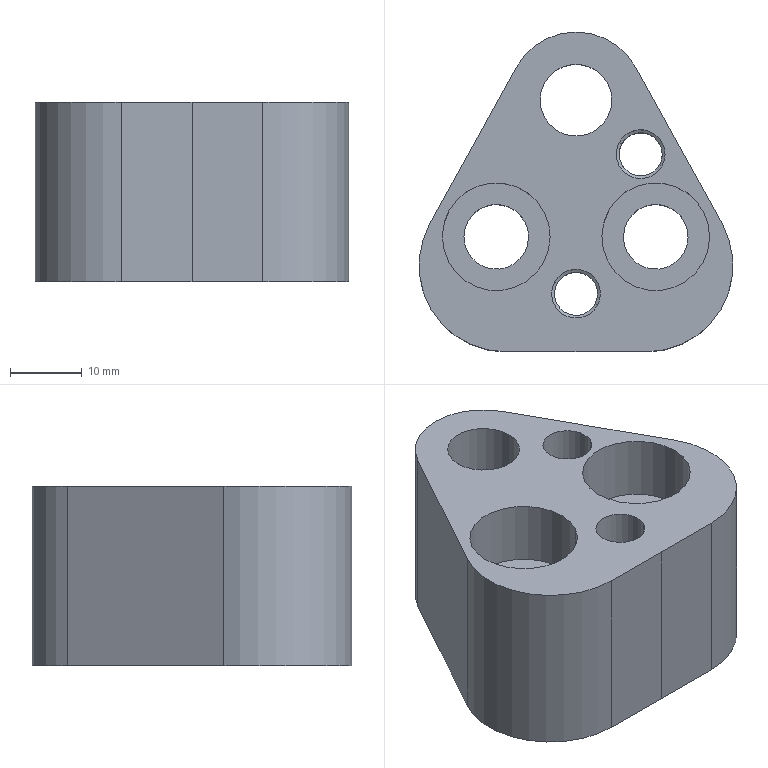Part | CATIA | 1 solid | 42 faces | box 43.7 x 44.5 x 25 mm | volume 25763 mm3 | cylinder 26 | plane 12 | cone 4 | commonest cylinder face diameters 6 x4 6.8 x4 9 x4 15 x4 5 x2 10 x2
STEP:
#1=CARTESIAN_POINT('',(2.984,-28.56,25.));
#2=VERTEX_POINT('',#1);
#3=CARTESIAN_POINT('',(-2.984,-25.3,25.));
#4=VERTEX_POINT('',#3);
#5=CARTESIAN_POINT('',(0.,-26.93,25.));
#6=DIRECTION('',(0.,0.,-1.));
#7=AXIS2_PLACEMENT_3D('',#5,#6,$);
#8=CIRCLE('',#7,3.4);
#9=EDGE_CURVE('',#2,#4,#8,.F.);
#10=ORIENTED_EDGE('',*,*,#9,.T.);
#11=CARTESIAN_POINT('',(-2.984,-25.3,16.));
#12=VERTEX_POINT('',#11);
#13=CARTESIAN_POINT('',(-2.984,-25.3,20.655));
#14=DIRECTION('',(0.,0.,-1.));
#15=VECTOR('',#14,1.);
#16=LINE('',#13,#15);
#17=EDGE_CURVE('',#12,#4,#16,.F.);
#18=ORIENTED_EDGE('',*,*,#17,.F.);
#19=CARTESIAN_POINT('',(2.984,-28.56,16.));
#20=VERTEX_POINT('',#19);
#21=CARTESIAN_POINT('',(0.,-26.93,16.));
#22=DIRECTION('',(0.,0.,-1.));
#23=AXIS2_PLACEMENT_3D('',#21,#22,$);
#24=CIRCLE('',#23,3.4);
#25=EDGE_CURVE('',#12,#20,#24,.T.);
#26=ORIENTED_EDGE('',*,*,#25,.T.);
#27=CARTESIAN_POINT('',(2.984,-28.56,20.655));
#28=DIRECTION('',(0.,0.,-1.));
#29=VECTOR('',#28,1.);
#30=LINE('',#27,#29);
#31=EDGE_CURVE('',#20,#2,#30,.F.);
#32=ORIENTED_EDGE('',*,*,#31,.T.);
#33=EDGE_LOOP('',(#10,#18,#26,#32));
#34=FACE_OUTER_BOUND('',#33,.T.);
#35=CARTESIAN_POINT('',(0.,-26.93,24.9));
#36=DIRECTION('',(0.,0.,-1.));
#37=DIRECTION('',(0.8776,-0.4794,0.));
#38=AXIS2_PLACEMENT_3D('',#35,#36,#37);
#39=CYLINDRICAL_SURFACE('',#38,3.4);
#40=ADVANCED_FACE('',(#34),#39,.F.);
#41=CARTESIAN_POINT('',(0.,-26.93,25.));
#42=DIRECTION('',(0.,0.,-1.));
#43=AXIS2_PLACEMENT_3D('',#41,#42,$);
#44=CIRCLE('',#43,3.4);
#45=EDGE_CURVE('',#4,#2,#44,.F.);
#46=ORIENTED_EDGE('',*,*,#45,.T.);
#47=ORIENTED_EDGE('',*,*,#31,.F.);
#48=CARTESIAN_POINT('',(0.,-26.93,16.));
#49=DIRECTION('',(0.,0.,-1.));
#50=AXIS2_PLACEMENT_3D('',#48,#49,$);
#51=CIRCLE('',#50,3.4);
#52=EDGE_CURVE('',#20,#12,#51,.T.);
#53=ORIENTED_EDGE('',*,*,#52,.T.);
#54=ORIENTED_EDGE('',*,*,#17,.T.);
#55=EDGE_LOOP('',(#46,#47,#53,#54));
#56=FACE_OUTER_BOUND('',#55,.T.);
#57=ADVANCED_FACE('',(#56),#39,.F.);
#58=CARTESIAN_POINT('',(-2.633,-25.492,15.769));
#59=VERTEX_POINT('',#58);
#60=CARTESIAN_POINT('',(3.,-26.93,15.769));
#61=VERTEX_POINT('',#60);
#62=CARTESIAN_POINT('',(0.,-26.93,15.769));
#63=DIRECTION('',(0.,0.,1.));
#64=AXIS2_PLACEMENT_3D('',#62,#63,$);
#65=CIRCLE('',#64,3.);
#66=EDGE_CURVE('',#59,#61,#65,.F.);
#67=ORIENTED_EDGE('',*,*,#66,.T.);
#68=CARTESIAN_POINT('',(2.633,-28.368,15.769));
#69=VERTEX_POINT('',#68);
#70=CARTESIAN_POINT('',(0.,-26.93,15.769));
#71=DIRECTION('',(0.,0.,1.));
#72=AXIS2_PLACEMENT_3D('',#70,#71,$);
#73=CIRCLE('',#72,3.);
#74=EDGE_CURVE('',#69,#61,#73,.T.);
#75=ORIENTED_EDGE('',*,*,#74,.F.);
#76=CARTESIAN_POINT('',(1.492,-27.745,15.019));
#77=DIRECTION('',(0.76,-0.4152,0.5));
#78=VECTOR('',#77,1.);
#79=LINE('',#76,#78);
#80=EDGE_CURVE('',#69,#20,#79,.T.);
#81=ORIENTED_EDGE('',*,*,#80,.T.);
#82=ORIENTED_EDGE('',*,*,#25,.F.);
#83=CARTESIAN_POINT('',(-1.492,-26.115,15.019));
#84=DIRECTION('',(-0.76,0.4152,0.5));
#85=VECTOR('',#84,1.);
#86=LINE('',#83,#85);
#87=EDGE_CURVE('',#59,#12,#86,.T.);
#88=ORIENTED_EDGE('',*,*,#87,.F.);
#89=EDGE_LOOP('',(#67,#75,#81,#82,#88));
#90=FACE_OUTER_BOUND('',#89,.T.);
#91=CARTESIAN_POINT('',(0.,-26.93,14.037));
#92=DIRECTION('',(0.,0.,1.));
#93=DIRECTION('',(0.8776,-0.4794,0.));
#94=AXIS2_PLACEMENT_3D('',#91,#92,#93);
#95=CONICAL_SURFACE('',#94,0.,1.047);
#96=ADVANCED_FACE('',(#90),#95,.F.);
#97=CARTESIAN_POINT('',(-3.,-26.93,15.769));
#98=VERTEX_POINT('',#97);
#99=CARTESIAN_POINT('',(0.,-26.93,15.769));
#100=DIRECTION('',(0.,0.,1.));
#101=AXIS2_PLACEMENT_3D('',#99,#100,$);
#102=CIRCLE('',#101,3.);
#103=EDGE_CURVE('',#69,#98,#102,.F.);
#104=ORIENTED_EDGE('',*,*,#103,.T.);
#105=CARTESIAN_POINT('',(0.,-26.93,15.769));
#106=DIRECTION('',(0.,0.,1.));
#107=AXIS2_PLACEMENT_3D('',#105,#106,$);
#108=CIRCLE('',#107,3.);
#109=EDGE_CURVE('',#59,#98,#108,.T.);
#110=ORIENTED_EDGE('',*,*,#109,.F.);
#111=ORIENTED_EDGE('',*,*,#87,.T.);
#112=ORIENTED_EDGE('',*,*,#52,.F.);
#113=ORIENTED_EDGE('',*,*,#80,.F.);
#114=EDGE_LOOP('',(#104,#110,#111,#112,#113));
#115=FACE_OUTER_BOUND('',#114,.T.);
#116=ADVANCED_FACE('',(#115),#95,.F.);
#117=ORIENTED_EDGE('',*,*,#66,.F.);
#118=ORIENTED_EDGE('',*,*,#109,.T.);
#119=CARTESIAN_POINT('',(-3.,-26.93,0.));
#120=VERTEX_POINT('',#119);
#121=CARTESIAN_POINT('',(-3.,-26.93,12.5));
#122=DIRECTION('',(0.,0.,1.));
#123=VECTOR('',#122,1.);
#124=LINE('',#121,#123);
#125=EDGE_CURVE('',#120,#98,#124,.T.);
#126=ORIENTED_EDGE('',*,*,#125,.F.);
#127=CARTESIAN_POINT('',(3.,-26.93,0.));
#128=VERTEX_POINT('',#127);
#129=CARTESIAN_POINT('',(0.,-26.93,0.));
#130=DIRECTION('',(0.,0.,1.));
#131=AXIS2_PLACEMENT_3D('',#129,#130,$);
#132=CIRCLE('',#131,3.);
#133=EDGE_CURVE('',#128,#120,#132,.T.);
#134=ORIENTED_EDGE('',*,*,#133,.F.);
#135=CARTESIAN_POINT('',(3.,-26.93,12.5));
#136=DIRECTION('',(0.,0.,1.));
#137=VECTOR('',#136,1.);
#138=LINE('',#135,#137);
#139=EDGE_CURVE('',#128,#61,#138,.T.);
#140=ORIENTED_EDGE('',*,*,#139,.T.);
#141=EDGE_LOOP('',(#117,#118,#126,#134,#140));
#142=FACE_OUTER_BOUND('',#141,.T.);
#143=CARTESIAN_POINT('',(0.,-26.93,12.5));
#144=DIRECTION('',(0.,0.,1.));
#145=DIRECTION('',(1.,0.,0.));
#146=AXIS2_PLACEMENT_3D('',#143,#144,#145);
#147=CYLINDRICAL_SURFACE('',#146,3.);
#148=ADVANCED_FACE('',(#142),#147,.F.);
#149=CARTESIAN_POINT('',(8.315,4.594,0.));
#150=VERTEX_POINT('',#149);
#151=CARTESIAN_POINT('',(8.315,4.594,25.));
#152=VERTEX_POINT('',#151);
#153=CARTESIAN_POINT('',(8.315,4.594,12.5));
#154=DIRECTION('',(0.,0.,1.));
#155=VECTOR('',#154,1.);
#156=LINE('',#153,#155);
#157=EDGE_CURVE('',#150,#152,#156,.T.);
#158=ORIENTED_EDGE('',*,*,#157,.F.);
#159=CARTESIAN_POINT('',(0.,9.5,0.));
#160=VERTEX_POINT('',#159);
#161=CARTESIAN_POINT('',(0.,0.,0.));
#162=DIRECTION('',(0.,0.,1.));
#163=AXIS2_PLACEMENT_3D('',#161,#162,$);
#164=CIRCLE('',#163,9.5);
#165=EDGE_CURVE('',#150,#160,#164,.T.);
#166=ORIENTED_EDGE('',*,*,#165,.T.);
#167=CARTESIAN_POINT('',(0.,9.5,25.));
#168=VERTEX_POINT('',#167);
#169=CARTESIAN_POINT('',(0.,9.5,12.5));
#170=DIRECTION('',(0.,0.,1.));
#171=VECTOR('',#170,1.);
#172=LINE('',#169,#171);
#173=EDGE_CURVE('',#160,#168,#172,.T.);
#174=ORIENTED_EDGE('',*,*,#173,.T.);
#175=CARTESIAN_POINT('',(0.,0.,25.));
#176=DIRECTION('',(0.,0.,1.));
#177=AXIS2_PLACEMENT_3D('',#175,#176,$);
#178=CIRCLE('',#177,9.5);
#179=EDGE_CURVE('',#152,#168,#178,.T.);
#180=ORIENTED_EDGE('',*,*,#179,.F.);
#181=EDGE_LOOP('',(#158,#166,#174,#180));
#182=FACE_OUTER_BOUND('',#181,.T.);
#183=CARTESIAN_POINT('',(0.,0.,12.5));
#184=DIRECTION('',(0.,0.,1.));
#185=DIRECTION('',(0.8753,0.4836,0.));
#186=AXIS2_PLACEMENT_3D('',#183,#184,#185);
#187=CYLINDRICAL_SURFACE('',#186,9.5);
#188=ADVANCED_FACE('',(#182),#187,.T.);
#189=ORIENTED_EDGE('',*,*,#173,.F.);
#190=CARTESIAN_POINT('',(-8.315,4.594,0.));
#191=VERTEX_POINT('',#190);
#192=CARTESIAN_POINT('',(0.,0.,0.));
#193=DIRECTION('',(0.,0.,1.));
#194=AXIS2_PLACEMENT_3D('',#192,#193,$);
#195=CIRCLE('',#194,9.5);
#196=EDGE_CURVE('',#160,#191,#195,.T.);
#197=ORIENTED_EDGE('',*,*,#196,.T.);
#198=CARTESIAN_POINT('',(-8.315,4.594,25.));
#199=VERTEX_POINT('',#198);
#200=CARTESIAN_POINT('',(-8.315,4.594,12.5));
#201=DIRECTION('',(0.,0.,1.));
#202=VECTOR('',#201,1.);
#203=LINE('',#200,#202);
#204=EDGE_CURVE('',#191,#199,#203,.T.);
#205=ORIENTED_EDGE('',*,*,#204,.T.);
#206=CARTESIAN_POINT('',(0.,0.,25.));
#207=DIRECTION('',(0.,0.,1.));
#208=AXIS2_PLACEMENT_3D('',#206,#207,$);
#209=CIRCLE('',#208,9.5);
#210=EDGE_CURVE('',#168,#199,#209,.T.);
#211=ORIENTED_EDGE('',*,*,#210,.F.);
#212=EDGE_LOOP('',(#189,#197,#205,#211));
#213=FACE_OUTER_BOUND('',#212,.T.);
#214=ADVANCED_FACE('',(#213),#187,.T.);
#215=ORIENTED_EDGE('',*,*,#204,.F.);
#216=CARTESIAN_POINT('',(-20.354,-17.197,0.));
#217=VERTEX_POINT('',#216);
#218=CARTESIAN_POINT('',(-14.335,-6.302,0.));
#219=DIRECTION('',(-0.4836,-0.8753,0.));
#220=VECTOR('',#219,1.);
#221=LINE('',#218,#220);
#222=EDGE_CURVE('',#191,#217,#221,.T.);
#223=ORIENTED_EDGE('',*,*,#222,.T.);
#224=CARTESIAN_POINT('',(-20.354,-17.197,25.));
#225=VERTEX_POINT('',#224);
#226=CARTESIAN_POINT('',(-20.354,-17.197,12.5));
#227=DIRECTION('',(0.,0.,1.));
#228=VECTOR('',#227,1.);
#229=LINE('',#226,#228);
#230=EDGE_CURVE('',#217,#225,#229,.T.);
#231=ORIENTED_EDGE('',*,*,#230,.T.);
#232=CARTESIAN_POINT('',(-14.335,-6.302,25.));
#233=DIRECTION('',(-0.4836,-0.8753,0.));
#234=VECTOR('',#233,1.);
#235=LINE('',#232,#234);
#236=EDGE_CURVE('',#199,#225,#235,.T.);
#237=ORIENTED_EDGE('',*,*,#236,.F.);
#238=EDGE_LOOP('',(#215,#223,#231,#237));
#239=FACE_OUTER_BOUND('',#238,.T.);
#240=CARTESIAN_POINT('',(-8.315,4.594,0.));
#241=DIRECTION('',(-0.8753,0.4836,0.));
#242=DIRECTION('',(-0.4836,-0.8753,0.));
#243=AXIS2_PLACEMENT_3D('',#240,#241,#242);
#244=PLANE('',#243);
#245=ADVANCED_FACE('',(#239),#244,.T.);
#246=ORIENTED_EDGE('',*,*,#230,.F.);
#247=CARTESIAN_POINT('',(-9.85,-35.,0.));
#248=VERTEX_POINT('',#247);
#249=CARTESIAN_POINT('',(-9.85,-23.,0.));
#250=DIRECTION('',(0.,0.,1.));
#251=AXIS2_PLACEMENT_3D('',#249,#250,$);
#252=CIRCLE('',#251,12.);
#253=EDGE_CURVE('',#217,#248,#252,.T.);
#254=ORIENTED_EDGE('',*,*,#253,.T.);
#255=CARTESIAN_POINT('',(-9.85,-35.,25.));
#256=VERTEX_POINT('',#255);
#257=CARTESIAN_POINT('',(-9.85,-35.,12.5));
#258=DIRECTION('',(0.,0.,1.));
#259=VECTOR('',#258,1.);
#260=LINE('',#257,#259);
#261=EDGE_CURVE('',#248,#256,#260,.T.);
#262=ORIENTED_EDGE('',*,*,#261,.T.);
#263=CARTESIAN_POINT('',(-9.85,-23.,25.));
#264=DIRECTION('',(0.,0.,1.));
#265=AXIS2_PLACEMENT_3D('',#263,#264,$);
#266=CIRCLE('',#265,12.);
#267=EDGE_CURVE('',#225,#256,#266,.T.);
#268=ORIENTED_EDGE('',*,*,#267,.F.);
#269=EDGE_LOOP('',(#246,#254,#262,#268));
#270=FACE_OUTER_BOUND('',#269,.T.);
#271=CARTESIAN_POINT('',(-9.85,-23.,12.5));
#272=DIRECTION('',(0.,0.,1.));
#273=DIRECTION('',(-0.8753,0.4836,0.));
#274=AXIS2_PLACEMENT_3D('',#271,#272,#273);
#275=CYLINDRICAL_SURFACE('',#274,12.);
#276=ADVANCED_FACE('',(#270),#275,.T.);
#277=ORIENTED_EDGE('',*,*,#261,.F.);
#278=CARTESIAN_POINT('',(0.,-35.,0.));
#279=VERTEX_POINT('',#278);
#280=CARTESIAN_POINT('',(-4.925,-35.,0.));
#281=DIRECTION('',(1.,0.,0.));
#282=VECTOR('',#281,1.);
#283=LINE('',#280,#282);
#284=EDGE_CURVE('',#248,#279,#283,.T.);
#285=ORIENTED_EDGE('',*,*,#284,.T.);
#286=CARTESIAN_POINT('',(0.,-35.,25.));
#287=VERTEX_POINT('',#286);
#288=CARTESIAN_POINT('',(0.,-35.,12.5));
#289=DIRECTION('',(0.,0.,1.));
#290=VECTOR('',#289,1.);
#291=LINE('',#288,#290);
#292=EDGE_CURVE('',#279,#287,#291,.T.);
#293=ORIENTED_EDGE('',*,*,#292,.T.);
#294=CARTESIAN_POINT('',(-4.925,-35.,25.));
#295=DIRECTION('',(1.,0.,0.));
#296=VECTOR('',#295,1.);
#297=LINE('',#294,#296);
#298=EDGE_CURVE('',#256,#287,#297,.T.);
#299=ORIENTED_EDGE('',*,*,#298,.F.);
#300=EDGE_LOOP('',(#277,#285,#293,#299));
#301=FACE_OUTER_BOUND('',#300,.T.);
#302=CARTESIAN_POINT('',(-9.85,-35.,0.));
#303=DIRECTION('',(0.,-1.,0.));
#304=DIRECTION('',(1.,0.,0.));
#305=AXIS2_PLACEMENT_3D('',#302,#303,#304);
#306=PLANE('',#305);
#307=ADVANCED_FACE('',(#301),#306,.T.);
#308=ORIENTED_EDGE('',*,*,#292,.F.);
#309=CARTESIAN_POINT('',(9.85,-35.,0.));
#310=VERTEX_POINT('',#309);
#311=CARTESIAN_POINT('',(4.925,-35.,0.));
#312=DIRECTION('',(-1.,0.,0.));
#313=VECTOR('',#312,1.);
#314=LINE('',#311,#313);
#315=EDGE_CURVE('',#279,#310,#314,.F.);
#316=ORIENTED_EDGE('',*,*,#315,.T.);
#317=CARTESIAN_POINT('',(9.85,-35.,25.));
#318=VERTEX_POINT('',#317);
#319=CARTESIAN_POINT('',(9.85,-35.,12.5));
#320=DIRECTION('',(0.,0.,1.));
#321=VECTOR('',#320,1.);
#322=LINE('',#319,#321);
#323=EDGE_CURVE('',#310,#318,#322,.T.);
#324=ORIENTED_EDGE('',*,*,#323,.T.);
#325=CARTESIAN_POINT('',(4.925,-35.,25.));
#326=DIRECTION('',(-1.,0.,0.));
#327=VECTOR('',#326,1.);
#328=LINE('',#325,#327);
#329=EDGE_CURVE('',#287,#318,#328,.F.);
#330=ORIENTED_EDGE('',*,*,#329,.F.);
#331=EDGE_LOOP('',(#308,#316,#324,#330));
#332=FACE_OUTER_BOUND('',#331,.T.);
#333=ADVANCED_FACE('',(#332),#306,.T.);
#334=ORIENTED_EDGE('',*,*,#323,.F.);
#335=CARTESIAN_POINT('',(20.354,-17.197,0.));
#336=VERTEX_POINT('',#335);
#337=CARTESIAN_POINT('',(9.85,-23.,0.));
#338=DIRECTION('',(0.,0.,1.));
#339=AXIS2_PLACEMENT_3D('',#337,#338,$);
#340=CIRCLE('',#339,12.);
#341=EDGE_CURVE('',#310,#336,#340,.T.);
#342=ORIENTED_EDGE('',*,*,#341,.T.);
#343=CARTESIAN_POINT('',(20.354,-17.197,25.));
#344=VERTEX_POINT('',#343);
#345=CARTESIAN_POINT('',(20.354,-17.197,12.5));
#346=DIRECTION('',(0.,0.,1.));
#347=VECTOR('',#346,1.);
#348=LINE('',#345,#347);
#349=EDGE_CURVE('',#336,#344,#348,.T.);
#350=ORIENTED_EDGE('',*,*,#349,.T.);
#351=CARTESIAN_POINT('',(9.85,-23.,25.));
#352=DIRECTION('',(0.,0.,1.));
#353=AXIS2_PLACEMENT_3D('',#351,#352,$);
#354=CIRCLE('',#353,12.);
#355=EDGE_CURVE('',#318,#344,#354,.T.);
#356=ORIENTED_EDGE('',*,*,#355,.F.);
#357=EDGE_LOOP('',(#334,#342,#350,#356));
#358=FACE_OUTER_BOUND('',#357,.T.);
#359=CARTESIAN_POINT('',(9.85,-23.,12.5));
#360=DIRECTION('',(0.,0.,1.));
#361=DIRECTION('',(0.,-1.,0.));
#362=AXIS2_PLACEMENT_3D('',#359,#360,#361);
#363=CYLINDRICAL_SURFACE('',#362,12.);
#364=ADVANCED_FACE('',(#358),#363,.T.);
#365=ORIENTED_EDGE('',*,*,#349,.F.);
#366=CARTESIAN_POINT('',(14.335,-6.302,0.));
#367=DIRECTION('',(0.4836,-0.8753,0.));
#368=VECTOR('',#367,1.);
#369=LINE('',#366,#368);
#370=EDGE_CURVE('',#336,#150,#369,.F.);
#371=ORIENTED_EDGE('',*,*,#370,.T.);
#372=ORIENTED_EDGE('',*,*,#157,.T.);
#373=CARTESIAN_POINT('',(14.335,-6.302,25.));
#374=DIRECTION('',(0.4836,-0.8753,0.));
#375=VECTOR('',#374,1.);
#376=LINE('',#373,#375);
#377=EDGE_CURVE('',#344,#152,#376,.F.);
#378=ORIENTED_EDGE('',*,*,#377,.F.);
#379=EDGE_LOOP('',(#365,#371,#372,#378));
#380=FACE_OUTER_BOUND('',#379,.T.);
#381=CARTESIAN_POINT('',(8.315,4.594,0.));
#382=DIRECTION('',(-0.8753,-0.4836,0.));
#383=DIRECTION('',(0.4836,-0.8753,0.));
#384=AXIS2_PLACEMENT_3D('',#381,#382,#383);
#385=PLANE('',#384);
#386=ADVANCED_FACE('',(#380),#385,.F.);
#387=CARTESIAN_POINT('',(17.682,-22.596,16.));
#388=VERTEX_POINT('',#387);
#389=CARTESIAN_POINT('',(4.518,-15.404,16.));
#390=VERTEX_POINT('',#389);
#391=CARTESIAN_POINT('',(11.1,-19.,16.));
#392=DIRECTION('',(0.,0.,-1.));
#393=AXIS2_PLACEMENT_3D('',#391,#392,$);
#394=CIRCLE('',#393,7.5);
#395=EDGE_CURVE('',#388,#390,#394,.T.);
#396=ORIENTED_EDGE('',*,*,#395,.F.);
#397=CARTESIAN_POINT('',(11.1,-19.,16.));
#398=DIRECTION('',(0.,0.,-1.));
#399=AXIS2_PLACEMENT_3D('',#397,#398,$);
#400=CIRCLE('',#399,7.5);
#401=EDGE_CURVE('',#390,#388,#400,.T.);
#402=ORIENTED_EDGE('',*,*,#401,.F.);
#403=EDGE_LOOP('',(#396,#402));
#404=FACE_OUTER_BOUND('',#403,.T.);
#405=CARTESIAN_POINT('',(7.151,-16.843,16.));
#406=VERTEX_POINT('',#405);
#407=CARTESIAN_POINT('',(15.049,-21.157,16.));
#408=VERTEX_POINT('',#407);
#409=CARTESIAN_POINT('',(11.1,-19.,16.));
#410=DIRECTION('',(0.,0.,-1.));
#411=AXIS2_PLACEMENT_3D('',#409,#410,$);
#412=CIRCLE('',#411,4.5);
#413=EDGE_CURVE('',#406,#408,#412,.T.);
#414=ORIENTED_EDGE('',*,*,#413,.T.);
#415=CARTESIAN_POINT('',(11.1,-19.,16.));
#416=DIRECTION('',(0.,0.,-1.));
#417=AXIS2_PLACEMENT_3D('',#415,#416,$);
#418=CIRCLE('',#417,4.5);
#419=EDGE_CURVE('',#408,#406,#418,.T.);
#420=ORIENTED_EDGE('',*,*,#419,.T.);
#421=EDGE_LOOP('',(#414,#420));
#422=FACE_BOUND('',#421,.T.);
#423=CARTESIAN_POINT('',(-6.6,-19.,16.));
#424=DIRECTION('',(0.,0.,-1.));
#425=DIRECTION('',(1.,0.,0.));
#426=AXIS2_PLACEMENT_3D('',#423,#424,#425);
#427=PLANE('',#426);
#428=ADVANCED_FACE('',(#404,#422),#427,.F.);
#429=CARTESIAN_POINT('',(7.151,-16.843,0.));
#430=VERTEX_POINT('',#429);
#431=CARTESIAN_POINT('',(15.049,-21.157,0.));
#432=VERTEX_POINT('',#431);
#433=CARTESIAN_POINT('',(11.1,-19.,0.));
#434=DIRECTION('',(0.,0.,-1.));
#435=AXIS2_PLACEMENT_3D('',#433,#434,$);
#436=CIRCLE('',#435,4.5);
#437=EDGE_CURVE('',#430,#432,#436,.F.);
#438=ORIENTED_EDGE('',*,*,#437,.F.);
#439=CARTESIAN_POINT('',(7.151,-16.843,7.8));
#440=DIRECTION('',(0.,0.,-1.));
#441=VECTOR('',#440,1.);
#442=LINE('',#439,#441);
#443=EDGE_CURVE('',#430,#406,#442,.F.);
#444=ORIENTED_EDGE('',*,*,#443,.T.);
#445=ORIENTED_EDGE('',*,*,#419,.F.);
#446=CARTESIAN_POINT('',(15.049,-21.157,7.8));
#447=DIRECTION('',(0.,0.,-1.));
#448=VECTOR('',#447,1.);
#449=LINE('',#446,#448);
#450=EDGE_CURVE('',#432,#408,#449,.F.);
#451=ORIENTED_EDGE('',*,*,#450,.F.);
#452=EDGE_LOOP('',(#438,#444,#445,#451));
#453=FACE_OUTER_BOUND('',#452,.T.);
#454=CARTESIAN_POINT('',(11.1,-19.,24.9));
#455=DIRECTION('',(0.,0.,-1.));
#456=DIRECTION('',(0.8776,-0.4794,0.));
#457=AXIS2_PLACEMENT_3D('',#454,#455,#456);
#458=CYLINDRICAL_SURFACE('',#457,4.5);
#459=ADVANCED_FACE('',(#453),#458,.F.);
#460=CARTESIAN_POINT('',(11.1,-19.,0.));
#461=DIRECTION('',(0.,0.,-1.));
#462=AXIS2_PLACEMENT_3D('',#460,#461,$);
#463=CIRCLE('',#462,4.5);
#464=EDGE_CURVE('',#432,#430,#463,.F.);
#465=ORIENTED_EDGE('',*,*,#464,.F.);
#466=ORIENTED_EDGE('',*,*,#450,.T.);
#467=ORIENTED_EDGE('',*,*,#413,.F.);
#468=ORIENTED_EDGE('',*,*,#443,.F.);
#469=EDGE_LOOP('',(#465,#466,#467,#468));
#470=FACE_OUTER_BOUND('',#469,.T.);
#471=ADVANCED_FACE('',(#470),#458,.F.);
#472=CARTESIAN_POINT('',(-4.518,-22.596,16.));
#473=VERTEX_POINT('',#472);
#474=CARTESIAN_POINT('',(-17.682,-15.404,16.));
#475=VERTEX_POINT('',#474);
#476=CARTESIAN_POINT('',(-11.1,-19.,16.));
#477=DIRECTION('',(0.,0.,-1.));
#478=AXIS2_PLACEMENT_3D('',#476,#477,$);
#479=CIRCLE('',#478,7.5);
#480=EDGE_CURVE('',#473,#475,#479,.T.);
#481=ORIENTED_EDGE('',*,*,#480,.F.);
#482=CARTESIAN_POINT('',(-11.1,-19.,16.));
#483=DIRECTION('',(0.,0.,-1.));
#484=AXIS2_PLACEMENT_3D('',#482,#483,$);
#485=CIRCLE('',#484,7.5);
#486=EDGE_CURVE('',#475,#473,#485,.T.);
#487=ORIENTED_EDGE('',*,*,#486,.F.);
#488=EDGE_LOOP('',(#481,#487));
#489=FACE_OUTER_BOUND('',#488,.T.);
#490=CARTESIAN_POINT('',(-15.049,-16.843,16.));
#491=VERTEX_POINT('',#490);
#492=CARTESIAN_POINT('',(-7.151,-21.157,16.));
#493=VERTEX_POINT('',#492);
#494=CARTESIAN_POINT('',(-11.1,-19.,16.));
#495=DIRECTION('',(0.,0.,-1.));
#496=AXIS2_PLACEMENT_3D('',#494,#495,$);
#497=CIRCLE('',#496,4.5);
#498=EDGE_CURVE('',#491,#493,#497,.T.);
#499=ORIENTED_EDGE('',*,*,#498,.T.);
#500=CARTESIAN_POINT('',(-11.1,-19.,16.));
#501=DIRECTION('',(0.,0.,-1.));
#502=AXIS2_PLACEMENT_3D('',#500,#501,$);
#503=CIRCLE('',#502,4.5);
#504=EDGE_CURVE('',#493,#491,#503,.T.);
#505=ORIENTED_EDGE('',*,*,#504,.T.);
#506=EDGE_LOOP('',(#499,#505));
#507=FACE_BOUND('',#506,.T.);
#508=ADVANCED_FACE('',(#489,#507),#427,.F.);
#509=CARTESIAN_POINT('',(-15.049,-16.843,0.));
#510=VERTEX_POINT('',#509);
#511=CARTESIAN_POINT('',(-7.151,-21.157,0.));
#512=VERTEX_POINT('',#511);
#513=CARTESIAN_POINT('',(-11.1,-19.,0.));
#514=DIRECTION('',(0.,0.,-1.));
#515=AXIS2_PLACEMENT_3D('',#513,#514,$);
#516=CIRCLE('',#515,4.5);
#517=EDGE_CURVE('',#510,#512,#516,.F.);
#518=ORIENTED_EDGE('',*,*,#517,.F.);
#519=CARTESIAN_POINT('',(-15.049,-16.843,7.8));
#520=DIRECTION('',(0.,0.,-1.));
#521=VECTOR('',#520,1.);
#522=LINE('',#519,#521);
#523=EDGE_CURVE('',#510,#491,#522,.F.);
#524=ORIENTED_EDGE('',*,*,#523,.T.);
#525=ORIENTED_EDGE('',*,*,#504,.F.);
#526=CARTESIAN_POINT('',(-7.151,-21.157,7.8));
#527=DIRECTION('',(0.,0.,-1.));
#528=VECTOR('',#527,1.);
#529=LINE('',#526,#528);
#530=EDGE_CURVE('',#512,#493,#529,.F.);
#531=ORIENTED_EDGE('',*,*,#530,.F.);
#532=EDGE_LOOP('',(#518,#524,#525,#531));
#533=FACE_OUTER_BOUND('',#532,.T.);
#534=CARTESIAN_POINT('',(-11.1,-19.,24.9));
#535=DIRECTION('',(0.,0.,-1.));
#536=DIRECTION('',(0.8776,-0.4794,0.));
#537=AXIS2_PLACEMENT_3D('',#534,#535,#536);
#538=CYLINDRICAL_SURFACE('',#537,4.5);
#539=ADVANCED_FACE('',(#533),#538,.F.);
#540=CARTESIAN_POINT('',(-11.1,-19.,0.));
#541=DIRECTION('',(0.,0.,-1.));
#542=AXIS2_PLACEMENT_3D('',#540,#541,$);
#543=CIRCLE('',#542,4.5);
#544=EDGE_CURVE('',#512,#510,#543,.F.);
#545=ORIENTED_EDGE('',*,*,#544,.F.);
#546=ORIENTED_EDGE('',*,*,#530,.T.);
#547=ORIENTED_EDGE('',*,*,#498,.F.);
#548=ORIENTED_EDGE('',*,*,#523,.F.);
#549=EDGE_LOOP('',(#545,#546,#547,#548));
#550=FACE_OUTER_BOUND('',#549,.T.);
#551=ADVANCED_FACE('',(#550),#538,.F.);
#552=CARTESIAN_POINT('',(-5.,4.5,0.));
#553=VERTEX_POINT('',#552);
#554=CARTESIAN_POINT('',(-5.,4.5,5.));
#555=VERTEX_POINT('',#554);
#556=CARTESIAN_POINT('',(-5.,4.5,2.5));
#557=DIRECTION('',(0.,0.,1.));
#558=VECTOR('',#557,1.);
#559=LINE('',#556,#558);
#560=EDGE_CURVE('',#553,#555,#559,.T.);
#561=ORIENTED_EDGE('',*,*,#560,.T.);
#562=CARTESIAN_POINT('',(-5.,0.,5.));
#563=VERTEX_POINT('',#562);
#564=CARTESIAN_POINT('',(-5.,2.25,5.));
#565=DIRECTION('',(0.,-1.,0.));
#566=VECTOR('',#565,1.);
#567=LINE('',#564,#566);
#568=EDGE_CURVE('',#555,#563,#567,.T.);
#569=ORIENTED_EDGE('',*,*,#568,.T.);
#570=CARTESIAN_POINT('',(-5.,-4.5,5.));
#571=VERTEX_POINT('',#570);
#572=CARTESIAN_POINT('',(-5.,-2.25,5.));
#573=DIRECTION('',(0.,-1.,0.));
#574=VECTOR('',#573,1.);
#575=LINE('',#572,#574);
#576=EDGE_CURVE('',#563,#571,#575,.T.);
#577=ORIENTED_EDGE('',*,*,#576,.T.);
#578=CARTESIAN_POINT('',(-5.,-4.5,0.));
#579=VERTEX_POINT('',#578);
#580=CARTESIAN_POINT('',(-5.,-4.5,2.5));
#581=DIRECTION('',(0.,0.,1.));
#582=VECTOR('',#581,1.);
#583=LINE('',#580,#582);
#584=EDGE_CURVE('',#579,#571,#583,.T.);
#585=ORIENTED_EDGE('',*,*,#584,.F.);
#586=CARTESIAN_POINT('',(-5.,0.,0.));
#587=DIRECTION('',(0.,-1.,0.));
#588=VECTOR('',#587,1.);
#589=LINE('',#586,#588);
#590=EDGE_CURVE('',#553,#579,#589,.T.);
#591=ORIENTED_EDGE('',*,*,#590,.F.);
#592=EDGE_LOOP('',(#561,#569,#577,#585,#591));
#593=FACE_OUTER_BOUND('',#592,.T.);
#594=CARTESIAN_POINT('',(-5.,4.5,0.));
#595=DIRECTION('',(-1.,0.,0.));
#596=DIRECTION('',(0.,-1.,0.));
#597=AXIS2_PLACEMENT_3D('',#594,#595,#596);
#598=PLANE('',#597);
#599=ADVANCED_FACE('',(#593),#598,.F.);
#600=CARTESIAN_POINT('',(-2.5,7.,5.));
#601=VERTEX_POINT('',#600);
#602=CARTESIAN_POINT('',(-2.5,4.5,5.));
#603=DIRECTION('',(0.,0.,1.));
#604=AXIS2_PLACEMENT_3D('',#602,#603,$);
#605=CIRCLE('',#604,2.5);
#606=EDGE_CURVE('',#601,#555,#605,.T.);
#607=ORIENTED_EDGE('',*,*,#606,.T.);
#608=ORIENTED_EDGE('',*,*,#560,.F.);
#609=CARTESIAN_POINT('',(-2.5,7.,0.));
#610=VERTEX_POINT('',#609);
#611=CARTESIAN_POINT('',(-2.5,4.5,0.));
#612=DIRECTION('',(0.,0.,1.));
#613=AXIS2_PLACEMENT_3D('',#611,#612,$);
#614=CIRCLE('',#613,2.5);
#615=EDGE_CURVE('',#610,#553,#614,.T.);
#616=ORIENTED_EDGE('',*,*,#615,.F.);
#617=CARTESIAN_POINT('',(-2.5,7.,2.5));
#618=DIRECTION('',(0.,0.,1.));
#619=VECTOR('',#618,1.);
#620=LINE('',#617,#619);
#621=EDGE_CURVE('',#610,#601,#620,.T.);
#622=ORIENTED_EDGE('',*,*,#621,.T.);
#623=EDGE_LOOP('',(#607,#608,#616,#622));
#624=FACE_OUTER_BOUND('',#623,.T.);
#625=CARTESIAN_POINT('',(-2.5,4.5,2.5));
#626=DIRECTION('',(0.,0.,1.));
#627=DIRECTION('',(0.,1.,0.));
#628=AXIS2_PLACEMENT_3D('',#625,#626,#627);
#629=CYLINDRICAL_SURFACE('',#628,2.5);
#630=ADVANCED_FACE('',(#624),#629,.F.);
#631=CARTESIAN_POINT('',(0.,7.,5.));
#632=VERTEX_POINT('',#631);
#633=CARTESIAN_POINT('',(-1.25,7.,5.));
#634=DIRECTION('',(-1.,0.,0.));
#635=VECTOR('',#634,1.);
#636=LINE('',#633,#635);
#637=EDGE_CURVE('',#632,#601,#636,.T.);
#638=ORIENTED_EDGE('',*,*,#637,.T.);
#639=ORIENTED_EDGE('',*,*,#621,.F.);
#640=CARTESIAN_POINT('',(0.,7.,0.));
#641=VERTEX_POINT('',#640);
#642=CARTESIAN_POINT('',(-1.25,7.,0.));
#643=DIRECTION('',(-1.,0.,0.));
#644=VECTOR('',#643,1.);
#645=LINE('',#642,#644);
#646=EDGE_CURVE('',#641,#610,#645,.T.);
#647=ORIENTED_EDGE('',*,*,#646,.F.);
#648=CARTESIAN_POINT('',(0.,7.,2.5));
#649=DIRECTION('',(0.,0.,1.));
#650=VECTOR('',#649,1.);
#651=LINE('',#648,#650);
#652=EDGE_CURVE('',#641,#632,#651,.T.);
#653=ORIENTED_EDGE('',*,*,#652,.T.);
#654=EDGE_LOOP('',(#638,#639,#647,#653));
#655=FACE_OUTER_BOUND('',#654,.T.);
#656=CARTESIAN_POINT('',(0.,7.,0.));
#657=DIRECTION('',(0.,1.,0.));
#658=DIRECTION('',(-1.,0.,0.));
#659=AXIS2_PLACEMENT_3D('',#656,#657,#658);
#660=PLANE('',#659);
#661=ADVANCED_FACE('',(#655),#660,.F.);
#662=CARTESIAN_POINT('',(7.,0.,5.));
#663=VERTEX_POINT('',#662);
#664=CARTESIAN_POINT('',(0.,0.,5.));
#665=DIRECTION('',(0.,0.,1.));
#666=AXIS2_PLACEMENT_3D('',#664,#665,$);
#667=CIRCLE('',#666,7.);
#668=EDGE_CURVE('',#663,#632,#667,.T.);
#669=ORIENTED_EDGE('',*,*,#668,.T.);
#670=ORIENTED_EDGE('',*,*,#652,.F.);
#671=CARTESIAN_POINT('',(7.,0.,0.));
#672=VERTEX_POINT('',#671);
#673=CARTESIAN_POINT('',(0.,0.,0.));
#674=DIRECTION('',(0.,0.,1.));
#675=AXIS2_PLACEMENT_3D('',#673,#674,$);
#676=CIRCLE('',#675,7.);
#677=EDGE_CURVE('',#672,#641,#676,.T.);
#678=ORIENTED_EDGE('',*,*,#677,.F.);
#679=CARTESIAN_POINT('',(7.,0.,2.5));
#680=DIRECTION('',(0.,0.,1.));
#681=VECTOR('',#680,1.);
#682=LINE('',#679,#681);
#683=EDGE_CURVE('',#672,#663,#682,.T.);
#684=ORIENTED_EDGE('',*,*,#683,.T.);
#685=EDGE_LOOP('',(#669,#670,#678,#684));
#686=FACE_OUTER_BOUND('',#685,.T.);
#687=CARTESIAN_POINT('',(0.,0.,2.5));
#688=DIRECTION('',(0.,0.,1.));
#689=DIRECTION('',(1.,0.,0.));
#690=AXIS2_PLACEMENT_3D('',#687,#688,#689);
#691=CYLINDRICAL_SURFACE('',#690,7.);
#692=ADVANCED_FACE('',(#686),#691,.F.);
#693=CARTESIAN_POINT('',(0.,-7.,5.));
#694=VERTEX_POINT('',#693);
#695=CARTESIAN_POINT('',(0.,0.,5.));
#696=DIRECTION('',(0.,0.,1.));
#697=AXIS2_PLACEMENT_3D('',#695,#696,$);
#698=CIRCLE('',#697,7.);
#699=EDGE_CURVE('',#694,#663,#698,.T.);
#700=ORIENTED_EDGE('',*,*,#699,.T.);
#701=ORIENTED_EDGE('',*,*,#683,.F.);
#702=CARTESIAN_POINT('',(0.,-7.,0.));
#703=VERTEX_POINT('',#702);
#704=CARTESIAN_POINT('',(0.,0.,0.));
#705=DIRECTION('',(0.,0.,1.));
#706=AXIS2_PLACEMENT_3D('',#704,#705,$);
#707=CIRCLE('',#706,7.);
#708=EDGE_CURVE('',#703,#672,#707,.T.);
#709=ORIENTED_EDGE('',*,*,#708,.F.);
#710=CARTESIAN_POINT('',(0.,-7.,2.5));
#711=DIRECTION('',(0.,0.,1.));
#712=VECTOR('',#711,1.);
#713=LINE('',#710,#712);
#714=EDGE_CURVE('',#703,#694,#713,.T.);
#715=ORIENTED_EDGE('',*,*,#714,.T.);
#716=EDGE_LOOP('',(#700,#701,#709,#715));
#717=FACE_OUTER_BOUND('',#716,.T.);
#718=CARTESIAN_POINT('',(0.,0.,2.5));
#719=DIRECTION('',(0.,0.,1.));
#720=DIRECTION('',(0.,-1.,0.));
#721=AXIS2_PLACEMENT_3D('',#718,#719,#720);
#722=CYLINDRICAL_SURFACE('',#721,7.);
#723=ADVANCED_FACE('',(#717),#722,.F.);
#724=CARTESIAN_POINT('',(-2.5,-7.,5.));
#725=VERTEX_POINT('',#724);
#726=CARTESIAN_POINT('',(-1.25,-7.,5.));
#727=DIRECTION('',(1.,0.,0.));
#728=VECTOR('',#727,1.);
#729=LINE('',#726,#728);
#730=EDGE_CURVE('',#725,#694,#729,.T.);
#731=ORIENTED_EDGE('',*,*,#730,.T.);
#732=ORIENTED_EDGE('',*,*,#714,.F.);
#733=CARTESIAN_POINT('',(-2.5,-7.,0.));
#734=VERTEX_POINT('',#733);
#735=CARTESIAN_POINT('',(-1.25,-7.,0.));
#736=DIRECTION('',(1.,0.,0.));
#737=VECTOR('',#736,1.);
#738=LINE('',#735,#737);
#739=EDGE_CURVE('',#734,#703,#738,.T.);
#740=ORIENTED_EDGE('',*,*,#739,.F.);
#741=CARTESIAN_POINT('',(-2.5,-7.,2.5));
#742=DIRECTION('',(0.,0.,1.));
#743=VECTOR('',#742,1.);
#744=LINE('',#741,#743);
#745=EDGE_CURVE('',#734,#725,#744,.T.);
#746=ORIENTED_EDGE('',*,*,#745,.T.);
#747=EDGE_LOOP('',(#731,#732,#740,#746));
#748=FACE_OUTER_BOUND('',#747,.T.);
#749=CARTESIAN_POINT('',(-2.5,-7.,0.));
#750=DIRECTION('',(0.,-1.,0.));
#751=DIRECTION('',(1.,0.,0.));
#752=AXIS2_PLACEMENT_3D('',#749,#750,#751);
#753=PLANE('',#752);
#754=ADVANCED_FACE('',(#748),#753,.F.);
#755=CARTESIAN_POINT('',(-2.5,-4.5,5.));
#756=DIRECTION('',(0.,0.,1.));
#757=AXIS2_PLACEMENT_3D('',#755,#756,$);
#758=CIRCLE('',#757,2.5);
#759=EDGE_CURVE('',#571,#725,#758,.T.);
#760=ORIENTED_EDGE('',*,*,#759,.T.);
#761=ORIENTED_EDGE('',*,*,#745,.F.);
#762=CARTESIAN_POINT('',(-2.5,-4.5,0.));
#763=DIRECTION('',(0.,0.,1.));
#764=AXIS2_PLACEMENT_3D('',#762,#763,$);
#765=CIRCLE('',#764,2.5);
#766=EDGE_CURVE('',#579,#734,#765,.T.);
#767=ORIENTED_EDGE('',*,*,#766,.F.);
#768=ORIENTED_EDGE('',*,*,#584,.T.);
#769=EDGE_LOOP('',(#760,#761,#767,#768));
#770=FACE_OUTER_BOUND('',#769,.T.);
#771=CARTESIAN_POINT('',(-2.5,-4.5,2.5));
#772=DIRECTION('',(0.,0.,1.));
#773=DIRECTION('',(-1.,0.,0.));
#774=AXIS2_PLACEMENT_3D('',#771,#772,#773);
#775=CYLINDRICAL_SURFACE('',#774,2.5);
#776=ADVANCED_FACE('',(#770),#775,.F.);
#777=CARTESIAN_POINT('',(5.,0.,5.));
#778=VERTEX_POINT('',#777);
#779=CARTESIAN_POINT('',(0.,0.,5.));
#780=DIRECTION('',(0.,0.,1.));
#781=AXIS2_PLACEMENT_3D('',#779,#780,$);
#782=CIRCLE('',#781,5.);
#783=EDGE_CURVE('',#563,#778,#782,.T.);
#784=ORIENTED_EDGE('',*,*,#783,.T.);
#785=CARTESIAN_POINT('',(0.,0.,5.));
#786=DIRECTION('',(0.,0.,1.));
#787=AXIS2_PLACEMENT_3D('',#785,#786,$);
#788=CIRCLE('',#787,5.);
#789=EDGE_CURVE('',#778,#563,#788,.T.);
#790=ORIENTED_EDGE('',*,*,#789,.T.);
#791=ORIENTED_EDGE('',*,*,#568,.F.);
#792=ORIENTED_EDGE('',*,*,#606,.F.);
#793=ORIENTED_EDGE('',*,*,#637,.F.);
#794=ORIENTED_EDGE('',*,*,#668,.F.);
#795=ORIENTED_EDGE('',*,*,#699,.F.);
#796=ORIENTED_EDGE('',*,*,#730,.F.);
#797=ORIENTED_EDGE('',*,*,#759,.F.);
#798=ORIENTED_EDGE('',*,*,#576,.F.);
#799=EDGE_LOOP('',(#784,#790,#791,#792,#793,#794,#795,#796,#797,#798));
#800=FACE_OUTER_BOUND('',#799,.T.);
#801=CARTESIAN_POINT('',(0.,0.,5.));
#802=DIRECTION('',(0.,0.,1.));
#803=DIRECTION('',(1.,0.,0.));
#804=AXIS2_PLACEMENT_3D('',#801,#802,#803);
#805=PLANE('',#804);
#806=ADVANCED_FACE('',(#800),#805,.F.);
#807=ORIENTED_EDGE('',*,*,#370,.F.);
#808=ORIENTED_EDGE('',*,*,#341,.F.);
#809=ORIENTED_EDGE('',*,*,#315,.F.);
#810=ORIENTED_EDGE('',*,*,#284,.F.);
#811=ORIENTED_EDGE('',*,*,#253,.F.);
#812=ORIENTED_EDGE('',*,*,#222,.F.);
#813=ORIENTED_EDGE('',*,*,#196,.F.);
#814=ORIENTED_EDGE('',*,*,#165,.F.);
#815=EDGE_LOOP('',(#807,#808,#809,#810,#811,#812,#813,#814));
#816=FACE_OUTER_BOUND('',#815,.T.);
#817=ORIENTED_EDGE('',*,*,#437,.T.);
#818=ORIENTED_EDGE('',*,*,#464,.T.);
#819=EDGE_LOOP('',(#817,#818));
#820=FACE_BOUND('',#819,.T.);
#821=ORIENTED_EDGE('',*,*,#517,.T.);
#822=ORIENTED_EDGE('',*,*,#544,.T.);
#823=EDGE_LOOP('',(#821,#822));
#824=FACE_BOUND('',#823,.T.);
#825=ORIENTED_EDGE('',*,*,#766,.T.);
#826=ORIENTED_EDGE('',*,*,#739,.T.);
#827=ORIENTED_EDGE('',*,*,#708,.T.);
#828=ORIENTED_EDGE('',*,*,#677,.T.);
#829=ORIENTED_EDGE('',*,*,#646,.T.);
#830=ORIENTED_EDGE('',*,*,#615,.T.);
#831=ORIENTED_EDGE('',*,*,#590,.T.);
#832=EDGE_LOOP('',(#825,#826,#827,#828,#829,#830,#831));
#833=FACE_BOUND('',#832,.T.);
#834=ORIENTED_EDGE('',*,*,#133,.T.);
#835=CARTESIAN_POINT('',(0.,-26.93,0.));
#836=DIRECTION('',(0.,0.,1.));
#837=AXIS2_PLACEMENT_3D('',#835,#836,$);
#838=CIRCLE('',#837,3.);
#839=EDGE_CURVE('',#120,#128,#838,.T.);
#840=ORIENTED_EDGE('',*,*,#839,.T.);
#841=EDGE_LOOP('',(#834,#840));
#842=FACE_BOUND('',#841,.T.);
#843=CARTESIAN_POINT('',(12.,-7.5,0.));
#844=VERTEX_POINT('',#843);
#845=CARTESIAN_POINT('',(6.,-7.5,0.));
#846=VERTEX_POINT('',#845);
#847=CARTESIAN_POINT('',(9.,-7.5,0.));
#848=DIRECTION('',(0.,0.,1.));
#849=AXIS2_PLACEMENT_3D('',#847,#848,$);
#850=CIRCLE('',#849,3.);
#851=EDGE_CURVE('',#844,#846,#850,.T.);
#852=ORIENTED_EDGE('',*,*,#851,.T.);
#853=CARTESIAN_POINT('',(9.,-7.5,0.));
#854=DIRECTION('',(0.,0.,1.));
#855=AXIS2_PLACEMENT_3D('',#853,#854,$);
#856=CIRCLE('',#855,3.);
#857=EDGE_CURVE('',#846,#844,#856,.T.);
#858=ORIENTED_EDGE('',*,*,#857,.T.);
#859=EDGE_LOOP('',(#852,#858));
#860=FACE_BOUND('',#859,.T.);
#861=CARTESIAN_POINT('',(0.,0.,0.));
#862=DIRECTION('',(0.,0.,1.));
#863=DIRECTION('',(1.,0.,0.));
#864=AXIS2_PLACEMENT_3D('',#861,#862,#863);
#865=PLANE('',#864);
#866=ADVANCED_FACE('',(#816,#820,#824,#833,#842,#860),#865,.F.);
#867=ORIENTED_EDGE('',*,*,#789,.F.);
#868=CARTESIAN_POINT('',(5.,0.,25.));
#869=VERTEX_POINT('',#868);
#870=CARTESIAN_POINT('',(5.,0.,12.5));
#871=DIRECTION('',(0.,0.,1.));
#872=VECTOR('',#871,1.);
#873=LINE('',#870,#872);
#874=EDGE_CURVE('',#778,#869,#873,.T.);
#875=ORIENTED_EDGE('',*,*,#874,.T.);
#876=CARTESIAN_POINT('',(-5.,0.,25.));
#877=VERTEX_POINT('',#876);
#878=CARTESIAN_POINT('',(0.,0.,25.));
#879=DIRECTION('',(0.,0.,1.));
#880=AXIS2_PLACEMENT_3D('',#878,#879,$);
#881=CIRCLE('',#880,5.);
#882=EDGE_CURVE('',#869,#877,#881,.T.);
#883=ORIENTED_EDGE('',*,*,#882,.T.);
#884=CARTESIAN_POINT('',(-5.,0.,12.5));
#885=DIRECTION('',(0.,0.,1.));
#886=VECTOR('',#885,1.);
#887=LINE('',#884,#886);
#888=EDGE_CURVE('',#563,#877,#887,.T.);
#889=ORIENTED_EDGE('',*,*,#888,.F.);
#890=EDGE_LOOP('',(#867,#875,#883,#889));
#891=FACE_OUTER_BOUND('',#890,.T.);
#892=CARTESIAN_POINT('',(0.,0.,12.5));
#893=DIRECTION('',(0.,0.,1.));
#894=DIRECTION('',(1.,0.,0.));
#895=AXIS2_PLACEMENT_3D('',#892,#893,#894);
#896=CYLINDRICAL_SURFACE('',#895,5.);
#897=ADVANCED_FACE('',(#891),#896,.F.);
#898=ORIENTED_EDGE('',*,*,#783,.F.);
#899=ORIENTED_EDGE('',*,*,#888,.T.);
#900=CARTESIAN_POINT('',(0.,0.,25.));
#901=DIRECTION('',(0.,0.,1.));
#902=AXIS2_PLACEMENT_3D('',#900,#901,$);
#903=CIRCLE('',#902,5.);
#904=EDGE_CURVE('',#877,#869,#903,.T.);
#905=ORIENTED_EDGE('',*,*,#904,.T.);
#906=ORIENTED_EDGE('',*,*,#874,.F.);
#907=EDGE_LOOP('',(#898,#899,#905,#906));
#908=FACE_OUTER_BOUND('',#907,.T.);
#909=ADVANCED_FACE('',(#908),#896,.F.);
#910=CARTESIAN_POINT('',(-4.518,-22.596,25.));
#911=VERTEX_POINT('',#910);
#912=CARTESIAN_POINT('',(-17.682,-15.404,25.));
#913=VERTEX_POINT('',#912);
#914=CARTESIAN_POINT('',(-11.1,-19.,25.));
#915=DIRECTION('',(0.,0.,-1.));
#916=AXIS2_PLACEMENT_3D('',#914,#915,$);
#917=CIRCLE('',#916,7.5);
#918=EDGE_CURVE('',#911,#913,#917,.F.);
#919=ORIENTED_EDGE('',*,*,#918,.T.);
#920=CARTESIAN_POINT('',(-17.682,-15.404,20.655));
#921=DIRECTION('',(0.,0.,-1.));
#922=VECTOR('',#921,1.);
#923=LINE('',#920,#922);
#924=EDGE_CURVE('',#475,#913,#923,.F.);
#925=ORIENTED_EDGE('',*,*,#924,.F.);
#926=ORIENTED_EDGE('',*,*,#486,.T.);
#927=CARTESIAN_POINT('',(-4.518,-22.596,20.655));
#928=DIRECTION('',(0.,0.,-1.));
#929=VECTOR('',#928,1.);
#930=LINE('',#927,#929);
#931=EDGE_CURVE('',#473,#911,#930,.F.);
#932=ORIENTED_EDGE('',*,*,#931,.T.);
#933=EDGE_LOOP('',(#919,#925,#926,#932));
#934=FACE_OUTER_BOUND('',#933,.T.);
#935=CARTESIAN_POINT('',(-11.1,-19.,24.9));
#936=DIRECTION('',(0.,0.,-1.));
#937=DIRECTION('',(0.8776,-0.4794,0.));
#938=AXIS2_PLACEMENT_3D('',#935,#936,#937);
#939=CYLINDRICAL_SURFACE('',#938,7.5);
#940=ADVANCED_FACE('',(#934),#939,.F.);
#941=CARTESIAN_POINT('',(-11.1,-19.,25.));
#942=DIRECTION('',(0.,0.,-1.));
#943=AXIS2_PLACEMENT_3D('',#941,#942,$);
#944=CIRCLE('',#943,7.5);
#945=EDGE_CURVE('',#913,#911,#944,.F.);
#946=ORIENTED_EDGE('',*,*,#945,.T.);
#947=ORIENTED_EDGE('',*,*,#931,.F.);
#948=ORIENTED_EDGE('',*,*,#480,.T.);
#949=ORIENTED_EDGE('',*,*,#924,.T.);
#950=EDGE_LOOP('',(#946,#947,#948,#949));
#951=FACE_OUTER_BOUND('',#950,.T.);
#952=ADVANCED_FACE('',(#951),#939,.F.);
#953=CARTESIAN_POINT('',(4.518,-15.404,25.));
#954=VERTEX_POINT('',#953);
#955=CARTESIAN_POINT('',(17.682,-22.596,25.));
#956=VERTEX_POINT('',#955);
#957=CARTESIAN_POINT('',(11.1,-19.,25.));
#958=DIRECTION('',(0.,0.,-1.));
#959=AXIS2_PLACEMENT_3D('',#957,#958,$);
#960=CIRCLE('',#959,7.5);
#961=EDGE_CURVE('',#954,#956,#960,.F.);
#962=ORIENTED_EDGE('',*,*,#961,.T.);
#963=CARTESIAN_POINT('',(17.682,-22.596,20.655));
#964=DIRECTION('',(0.,0.,-1.));
#965=VECTOR('',#964,1.);
#966=LINE('',#963,#965);
#967=EDGE_CURVE('',#388,#956,#966,.F.);
#968=ORIENTED_EDGE('',*,*,#967,.F.);
#969=ORIENTED_EDGE('',*,*,#395,.T.);
#970=CARTESIAN_POINT('',(4.518,-15.404,20.655));
#971=DIRECTION('',(0.,0.,-1.));
#972=VECTOR('',#971,1.);
#973=LINE('',#970,#972);
#974=EDGE_CURVE('',#390,#954,#973,.F.);
#975=ORIENTED_EDGE('',*,*,#974,.T.);
#976=EDGE_LOOP('',(#962,#968,#969,#975));
#977=FACE_OUTER_BOUND('',#976,.T.);
#978=CARTESIAN_POINT('',(11.1,-19.,24.9));
#979=DIRECTION('',(0.,0.,-1.));
#980=DIRECTION('',(0.8776,-0.4794,0.));
#981=AXIS2_PLACEMENT_3D('',#978,#979,#980);
#982=CYLINDRICAL_SURFACE('',#981,7.5);
#983=ADVANCED_FACE('',(#977),#982,.F.);
#984=CARTESIAN_POINT('',(11.1,-19.,25.));
#985=DIRECTION('',(0.,0.,-1.));
#986=AXIS2_PLACEMENT_3D('',#984,#985,$);
#987=CIRCLE('',#986,7.5);
#988=EDGE_CURVE('',#956,#954,#987,.F.);
#989=ORIENTED_EDGE('',*,*,#988,.T.);
#990=ORIENTED_EDGE('',*,*,#974,.F.);
#991=ORIENTED_EDGE('',*,*,#401,.T.);
#992=ORIENTED_EDGE('',*,*,#967,.T.);
#993=EDGE_LOOP('',(#989,#990,#991,#992));
#994=FACE_OUTER_BOUND('',#993,.T.);
#995=ADVANCED_FACE('',(#994),#982,.F.);
#996=ORIENTED_EDGE('',*,*,#103,.F.);
#997=ORIENTED_EDGE('',*,*,#74,.T.);
#998=ORIENTED_EDGE('',*,*,#139,.F.);
#999=ORIENTED_EDGE('',*,*,#839,.F.);
#1000=ORIENTED_EDGE('',*,*,#125,.T.);
#1001=EDGE_LOOP('',(#996,#997,#998,#999,#1000));
#1002=FACE_OUTER_BOUND('',#1001,.T.);
#1003=ADVANCED_FACE('',(#1002),#147,.F.);
#1004=CARTESIAN_POINT('',(11.633,-8.938,15.769));
#1005=VERTEX_POINT('',#1004);
#1006=CARTESIAN_POINT('',(6.,-7.5,15.769));
#1007=VERTEX_POINT('',#1006);
#1008=CARTESIAN_POINT('',(9.,-7.5,15.769));
#1009=DIRECTION('',(0.,0.,1.));
#1010=AXIS2_PLACEMENT_3D('',#1008,#1009,$);
#1011=CIRCLE('',#1010,3.);
#1012=EDGE_CURVE('',#1005,#1007,#1011,.F.);
#1013=ORIENTED_EDGE('',*,*,#1012,.F.);
#1014=CARTESIAN_POINT('',(12.,-7.5,15.769));
#1015=VERTEX_POINT('',#1014);
#1016=CARTESIAN_POINT('',(9.,-7.5,15.769));
#1017=DIRECTION('',(0.,0.,1.));
#1018=AXIS2_PLACEMENT_3D('',#1016,#1017,$);
#1019=CIRCLE('',#1018,3.);
#1020=EDGE_CURVE('',#1005,#1015,#1019,.T.);
#1021=ORIENTED_EDGE('',*,*,#1020,.T.);
#1022=CARTESIAN_POINT('',(12.,-7.5,12.5));
#1023=DIRECTION('',(0.,0.,1.));
#1024=VECTOR('',#1023,1.);
#1025=LINE('',#1022,#1024);
#1026=EDGE_CURVE('',#844,#1015,#1025,.T.);
#1027=ORIENTED_EDGE('',*,*,#1026,.F.);
#1028=ORIENTED_EDGE('',*,*,#857,.F.);
#1029=CARTESIAN_POINT('',(6.,-7.5,12.5));
#1030=DIRECTION('',(0.,0.,1.));
#1031=VECTOR('',#1030,1.);
#1032=LINE('',#1029,#1031);
#1033=EDGE_CURVE('',#846,#1007,#1032,.T.);
#1034=ORIENTED_EDGE('',*,*,#1033,.T.);
#1035=EDGE_LOOP('',(#1013,#1021,#1027,#1028,#1034));
#1036=FACE_OUTER_BOUND('',#1035,.T.);
#1037=CARTESIAN_POINT('',(9.,-7.5,12.5));
#1038=DIRECTION('',(0.,0.,1.));
#1039=DIRECTION('',(1.,0.,0.));
#1040=AXIS2_PLACEMENT_3D('',#1037,#1038,#1039);
#1041=CYLINDRICAL_SURFACE('',#1040,3.);
#1042=ADVANCED_FACE('',(#1036),#1041,.F.);
#1043=CARTESIAN_POINT('',(6.367,-6.062,15.769));
#1044=VERTEX_POINT('',#1043);
#1045=CARTESIAN_POINT('',(9.,-7.5,15.769));
#1046=DIRECTION('',(0.,0.,1.));
#1047=AXIS2_PLACEMENT_3D('',#1045,#1046,$);
#1048=CIRCLE('',#1047,3.);
#1049=EDGE_CURVE('',#1044,#1015,#1048,.F.);
#1050=ORIENTED_EDGE('',*,*,#1049,.F.);
#1051=CARTESIAN_POINT('',(9.,-7.5,15.769));
#1052=DIRECTION('',(0.,0.,1.));
#1053=AXIS2_PLACEMENT_3D('',#1051,#1052,$);
#1054=CIRCLE('',#1053,3.);
#1055=EDGE_CURVE('',#1044,#1007,#1054,.T.);
#1056=ORIENTED_EDGE('',*,*,#1055,.T.);
#1057=ORIENTED_EDGE('',*,*,#1033,.F.);
#1058=ORIENTED_EDGE('',*,*,#851,.F.);
#1059=ORIENTED_EDGE('',*,*,#1026,.T.);
#1060=EDGE_LOOP('',(#1050,#1056,#1057,#1058,#1059));
#1061=FACE_OUTER_BOUND('',#1060,.T.);
#1062=ADVANCED_FACE('',(#1061),#1041,.F.);
#1063=ORIENTED_EDGE('',*,*,#179,.T.);
#1064=ORIENTED_EDGE('',*,*,#210,.T.);
#1065=ORIENTED_EDGE('',*,*,#236,.T.);
#1066=ORIENTED_EDGE('',*,*,#267,.T.);
#1067=ORIENTED_EDGE('',*,*,#298,.T.);
#1068=ORIENTED_EDGE('',*,*,#329,.T.);
#1069=ORIENTED_EDGE('',*,*,#355,.T.);
#1070=ORIENTED_EDGE('',*,*,#377,.T.);
#1071=EDGE_LOOP('',(#1063,#1064,#1065,#1066,#1067,#1068,#1069,#1070));
#1072=FACE_OUTER_BOUND('',#1071,.T.);
#1073=CARTESIAN_POINT('',(11.984,-9.13,25.));
#1074=VERTEX_POINT('',#1073);
#1075=CARTESIAN_POINT('',(6.016,-5.87,25.));
#1076=VERTEX_POINT('',#1075);
#1077=CARTESIAN_POINT('',(9.,-7.5,25.));
#1078=DIRECTION('',(0.,0.,1.));
#1079=AXIS2_PLACEMENT_3D('',#1077,#1078,$);
#1080=CIRCLE('',#1079,3.4);
#1081=EDGE_CURVE('',#1074,#1076,#1080,.T.);
#1082=ORIENTED_EDGE('',*,*,#1081,.F.);
#1083=CARTESIAN_POINT('',(9.,-7.5,25.));
#1084=DIRECTION('',(0.,0.,1.));
#1085=AXIS2_PLACEMENT_3D('',#1083,#1084,$);
#1086=CIRCLE('',#1085,3.4);
#1087=EDGE_CURVE('',#1076,#1074,#1086,.T.);
#1088=ORIENTED_EDGE('',*,*,#1087,.F.);
#1089=EDGE_LOOP('',(#1082,#1088));
#1090=FACE_BOUND('',#1089,.T.);
#1091=ORIENTED_EDGE('',*,*,#45,.F.);
#1092=ORIENTED_EDGE('',*,*,#9,.F.);
#1093=EDGE_LOOP('',(#1091,#1092));
#1094=FACE_BOUND('',#1093,.T.);
#1095=ORIENTED_EDGE('',*,*,#988,.F.);
#1096=ORIENTED_EDGE('',*,*,#961,.F.);
#1097=EDGE_LOOP('',(#1095,#1096));
#1098=FACE_BOUND('',#1097,.T.);
#1099=ORIENTED_EDGE('',*,*,#945,.F.);
#1100=ORIENTED_EDGE('',*,*,#918,.F.);
#1101=EDGE_LOOP('',(#1099,#1100));
#1102=FACE_BOUND('',#1101,.T.);
#1103=ORIENTED_EDGE('',*,*,#904,.F.);
#1104=ORIENTED_EDGE('',*,*,#882,.F.);
#1105=EDGE_LOOP('',(#1103,#1104));
#1106=FACE_BOUND('',#1105,.T.);
#1107=CARTESIAN_POINT('',(0.,0.,25.));
#1108=DIRECTION('',(0.,0.,1.));
#1109=DIRECTION('',(1.,0.,0.));
#1110=AXIS2_PLACEMENT_3D('',#1107,#1108,#1109);
#1111=PLANE('',#1110);
#1112=ADVANCED_FACE('',(#1072,#1090,#1094,#1098,#1102,#1106),#1111,.T.);
#1113=ORIENTED_EDGE('',*,*,#1081,.T.);
#1114=CARTESIAN_POINT('',(6.016,-5.87,16.));
#1115=VERTEX_POINT('',#1114);
#1116=CARTESIAN_POINT('',(6.016,-5.87,20.655));
#1117=DIRECTION('',(0.,0.,-1.));
#1118=VECTOR('',#1117,1.);
#1119=LINE('',#1116,#1118);
#1120=EDGE_CURVE('',#1115,#1076,#1119,.F.);
#1121=ORIENTED_EDGE('',*,*,#1120,.F.);
#1122=CARTESIAN_POINT('',(11.984,-9.13,16.));
#1123=VERTEX_POINT('',#1122);
#1124=CARTESIAN_POINT('',(9.,-7.5,16.));
#1125=DIRECTION('',(0.,0.,-1.));
#1126=AXIS2_PLACEMENT_3D('',#1124,#1125,$);
#1127=CIRCLE('',#1126,3.4);
#1128=EDGE_CURVE('',#1115,#1123,#1127,.T.);
#1129=ORIENTED_EDGE('',*,*,#1128,.T.);
#1130=CARTESIAN_POINT('',(11.984,-9.13,20.655));
#1131=DIRECTION('',(0.,0.,-1.));
#1132=VECTOR('',#1131,1.);
#1133=LINE('',#1130,#1132);
#1134=EDGE_CURVE('',#1123,#1074,#1133,.F.);
#1135=ORIENTED_EDGE('',*,*,#1134,.T.);
#1136=EDGE_LOOP('',(#1113,#1121,#1129,#1135));
#1137=FACE_OUTER_BOUND('',#1136,.T.);
#1138=CARTESIAN_POINT('',(9.,-7.5,24.9));
#1139=DIRECTION('',(0.,0.,-1.));
#1140=DIRECTION('',(0.8776,-0.4794,0.));
#1141=AXIS2_PLACEMENT_3D('',#1138,#1139,#1140);
#1142=CYLINDRICAL_SURFACE('',#1141,3.4);
#1143=ADVANCED_FACE('',(#1137),#1142,.F.);
#1144=ORIENTED_EDGE('',*,*,#1087,.T.);
#1145=ORIENTED_EDGE('',*,*,#1134,.F.);
#1146=CARTESIAN_POINT('',(9.,-7.5,16.));
#1147=DIRECTION('',(0.,0.,-1.));
#1148=AXIS2_PLACEMENT_3D('',#1146,#1147,$);
#1149=CIRCLE('',#1148,3.4);
#1150=EDGE_CURVE('',#1123,#1115,#1149,.T.);
#1151=ORIENTED_EDGE('',*,*,#1150,.T.);
#1152=ORIENTED_EDGE('',*,*,#1120,.T.);
#1153=EDGE_LOOP('',(#1144,#1145,#1151,#1152));
#1154=FACE_OUTER_BOUND('',#1153,.T.);
#1155=ADVANCED_FACE('',(#1154),#1142,.F.);
#1156=ORIENTED_EDGE('',*,*,#1049,.T.);
#1157=ORIENTED_EDGE('',*,*,#1020,.F.);
#1158=CARTESIAN_POINT('',(10.492,-8.315,15.019));
#1159=DIRECTION('',(0.76,-0.4152,0.5));
#1160=VECTOR('',#1159,1.);
#1161=LINE('',#1158,#1160);
#1162=EDGE_CURVE('',#1005,#1123,#1161,.T.);
#1163=ORIENTED_EDGE('',*,*,#1162,.T.);
#1164=ORIENTED_EDGE('',*,*,#1128,.F.);
#1165=CARTESIAN_POINT('',(7.508,-6.685,15.019));
#1166=DIRECTION('',(-0.76,0.4152,0.5));
#1167=VECTOR('',#1166,1.);
#1168=LINE('',#1165,#1167);
#1169=EDGE_CURVE('',#1044,#1115,#1168,.T.);
#1170=ORIENTED_EDGE('',*,*,#1169,.F.);
#1171=EDGE_LOOP('',(#1156,#1157,#1163,#1164,#1170));
#1172=FACE_OUTER_BOUND('',#1171,.T.);
#1173=CARTESIAN_POINT('',(9.,-7.5,14.037));
#1174=DIRECTION('',(0.,0.,1.));
#1175=DIRECTION('',(0.8776,-0.4794,0.));
#1176=AXIS2_PLACEMENT_3D('',#1173,#1174,#1175);
#1177=CONICAL_SURFACE('',#1176,0.,1.047);
#1178=ADVANCED_FACE('',(#1172),#1177,.F.);
#1179=ORIENTED_EDGE('',*,*,#1012,.T.);
#1180=ORIENTED_EDGE('',*,*,#1055,.F.);
#1181=ORIENTED_EDGE('',*,*,#1169,.T.);
#1182=ORIENTED_EDGE('',*,*,#1150,.F.);
#1183=ORIENTED_EDGE('',*,*,#1162,.F.);
#1184=EDGE_LOOP('',(#1179,#1180,#1181,#1182,#1183));
#1185=FACE_OUTER_BOUND('',#1184,.T.);
#1186=ADVANCED_FACE('',(#1185),#1177,.F.);
#1187=CLOSED_SHELL('',(#40,#57,#96,#116,#148,#188,#214,#245,#276,#307,#333,#364,#386,#428,#459,#471,#508,#539,#551,#599,#630,#661,#692,#723,#754,#776,#806,#866,#897,#909,#940,#952,#983,#995,#1003,#1042,#1062,#1112,#1143,#1155,#1178,#1186));
#1188=MANIFOLD_SOLID_BREP('',#1187);
#1189=(LENGTH_UNIT()NAMED_UNIT(*)SI_UNIT(.MILLI.,.METRE.));
#1190=UNCERTAINTY_MEASURE_WITH_UNIT(LENGTH_MEASURE(0.005),#1189,'','');
#1191=(NAMED_UNIT(*)PLANE_ANGLE_UNIT()SI_UNIT($,.RADIAN.));
#1192=(NAMED_UNIT(*)SI_UNIT($,.STERADIAN.)SOLID_ANGLE_UNIT());
#1193=(GEOMETRIC_REPRESENTATION_CONTEXT(3)GLOBAL_UNCERTAINTY_ASSIGNED_CONTEXT((#1190))GLOBAL_UNIT_ASSIGNED_CONTEXT((#1189,#1191,#1192))REPRESENTATION_CONTEXT('',''));
#1194=ADVANCED_BREP_SHAPE_REPRESENTATION('',(#1188),#1193);